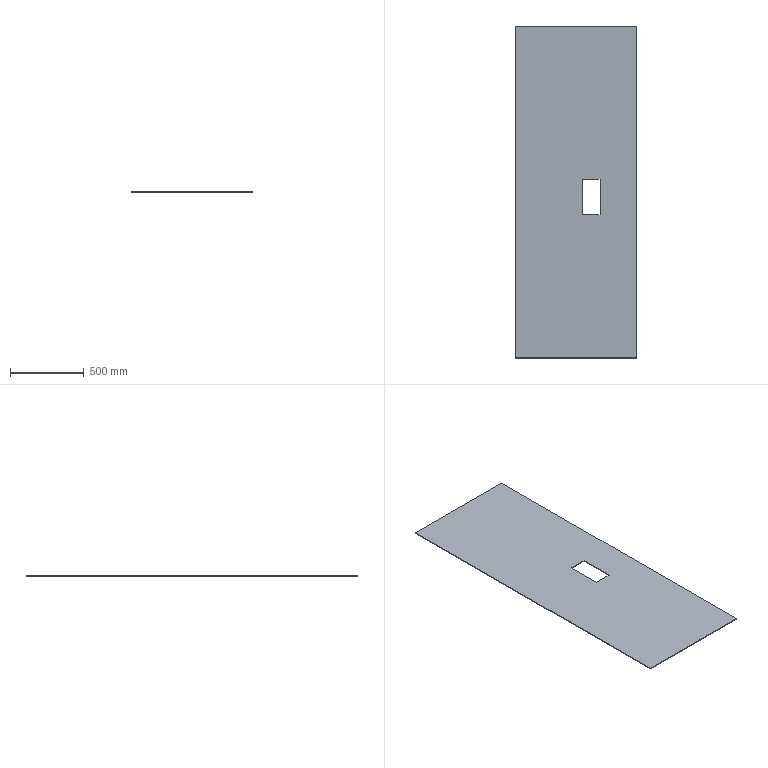Part | 1 solid | 10 faces | box 826 x 2252 x 5 mm | volume 9156760 mm3 | plane 10
STEP:
#1=CARTESIAN_POINT('',(-413.,1126.,5.));
#2=VERTEX_POINT('',#1);
#3=CARTESIAN_POINT('',(-413.,-1126.,5.));
#4=VERTEX_POINT('',#3);
#5=CARTESIAN_POINT('',(-413.,0.,5.));
#6=DIRECTION('',(0.,-1.,0.));
#7=VECTOR('',#6,1000.);
#8=LINE('',#5,#7);
#9=EDGE_CURVE('',#2,#4,#8,.T.);
#10=ORIENTED_EDGE('',*,*,#9,.T.);
#11=CARTESIAN_POINT('',(413.,-1126.,5.));
#12=VERTEX_POINT('',#11);
#13=CARTESIAN_POINT('',(0.,-1126.,5.));
#14=DIRECTION('',(1.,0.,0.));
#15=VECTOR('',#14,1000.);
#16=LINE('',#13,#15);
#17=EDGE_CURVE('',#4,#12,#16,.T.);
#18=ORIENTED_EDGE('',*,*,#17,.T.);
#19=CARTESIAN_POINT('',(413.,1126.,5.));
#20=VERTEX_POINT('',#19);
#21=CARTESIAN_POINT('',(413.,0.,5.));
#22=DIRECTION('',(0.,1.,0.));
#23=VECTOR('',#22,1000.);
#24=LINE('',#21,#23);
#25=EDGE_CURVE('',#12,#20,#24,.T.);
#26=ORIENTED_EDGE('',*,*,#25,.T.);
#27=CARTESIAN_POINT('',(0.,1126.,5.));
#28=DIRECTION('',(-1.,0.,0.));
#29=VECTOR('',#28,1000.);
#30=LINE('',#27,#29);
#31=EDGE_CURVE('',#20,#2,#30,.T.);
#32=ORIENTED_EDGE('',*,*,#31,.T.);
#33=EDGE_LOOP('',(#10,#18,#26,#32));
#34=FACE_OUTER_BOUND('',#33,.T.);
#35=CARTESIAN_POINT('',(163.,86.,5.));
#36=VERTEX_POINT('',#35);
#37=CARTESIAN_POINT('',(163.,-154.,5.));
#38=VERTEX_POINT('',#37);
#39=CARTESIAN_POINT('',(163.,0.,5.));
#40=DIRECTION('',(0.,-1.,0.));
#41=VECTOR('',#40,1000.);
#42=LINE('',#39,#41);
#43=EDGE_CURVE('',#36,#38,#42,.T.);
#44=ORIENTED_EDGE('',*,*,#43,.T.);
#45=CARTESIAN_POINT('',(43.,-154.,5.));
#46=VERTEX_POINT('',#45);
#47=CARTESIAN_POINT('',(0.,-154.,5.));
#48=DIRECTION('',(-1.,0.,0.));
#49=VECTOR('',#48,1000.);
#50=LINE('',#47,#49);
#51=EDGE_CURVE('',#38,#46,#50,.T.);
#52=ORIENTED_EDGE('',*,*,#51,.T.);
#53=CARTESIAN_POINT('',(43.,86.,5.));
#54=VERTEX_POINT('',#53);
#55=CARTESIAN_POINT('',(43.,0.,5.));
#56=DIRECTION('',(0.,1.,0.));
#57=VECTOR('',#56,1000.);
#58=LINE('',#55,#57);
#59=EDGE_CURVE('',#46,#54,#58,.T.);
#60=ORIENTED_EDGE('',*,*,#59,.T.);
#61=CARTESIAN_POINT('',(0.,86.,5.));
#62=DIRECTION('',(1.,0.,0.));
#63=VECTOR('',#62,1000.);
#64=LINE('',#61,#63);
#65=EDGE_CURVE('',#54,#36,#64,.T.);
#66=ORIENTED_EDGE('',*,*,#65,.T.);
#67=EDGE_LOOP('',(#44,#52,#60,#66));
#68=FACE_BOUND('',#67,.T.);
#69=CARTESIAN_POINT('',(0.,0.,5.));
#70=DIRECTION('',(0.,0.,1.));
#71=DIRECTION('',(1.,0.,0.));
#72=AXIS2_PLACEMENT_3D('',#69,#70,#71);
#73=PLANE('',#72);
#74=ADVANCED_FACE('',(#34,#68),#73,.T.);
#75=CARTESIAN_POINT('',(413.,-1126.,0.));
#76=VERTEX_POINT('',#75);
#77=CARTESIAN_POINT('',(413.,-1126.,5.));
#78=DIRECTION('',(0.,0.,-1.));
#79=VECTOR('',#78,1000.);
#80=LINE('',#77,#79);
#81=EDGE_CURVE('',#12,#76,#80,.T.);
#82=ORIENTED_EDGE('',*,*,#81,.F.);
#83=ORIENTED_EDGE('',*,*,#17,.F.);
#84=CARTESIAN_POINT('',(-413.,-1126.,0.));
#85=VERTEX_POINT('',#84);
#86=CARTESIAN_POINT('',(-413.,-1126.,5.));
#87=DIRECTION('',(0.,0.,1.));
#88=VECTOR('',#87,1000.);
#89=LINE('',#86,#88);
#90=EDGE_CURVE('',#85,#4,#89,.T.);
#91=ORIENTED_EDGE('',*,*,#90,.F.);
#92=CARTESIAN_POINT('',(-413.,-1126.,0.));
#93=DIRECTION('',(-1.,0.,0.));
#94=VECTOR('',#93,1000.);
#95=LINE('',#92,#94);
#96=EDGE_CURVE('',#76,#85,#95,.T.);
#97=ORIENTED_EDGE('',*,*,#96,.F.);
#98=EDGE_LOOP('',(#82,#83,#91,#97));
#99=FACE_OUTER_BOUND('',#98,.T.);
#100=CARTESIAN_POINT('',(-413.,-1126.,5.));
#101=DIRECTION('',(0.,1.,0.));
#102=DIRECTION('',(0.,0.,1.));
#103=AXIS2_PLACEMENT_3D('',#100,#101,#102);
#104=PLANE('',#103);
#105=ADVANCED_FACE('',(#99),#104,.F.);
#106=ORIENTED_EDGE('',*,*,#90,.T.);
#107=ORIENTED_EDGE('',*,*,#9,.F.);
#108=CARTESIAN_POINT('',(-413.,1126.,0.));
#109=VERTEX_POINT('',#108);
#110=CARTESIAN_POINT('',(-413.,1126.,5.));
#111=DIRECTION('',(0.,0.,1.));
#112=VECTOR('',#111,1000.);
#113=LINE('',#110,#112);
#114=EDGE_CURVE('',#109,#2,#113,.T.);
#115=ORIENTED_EDGE('',*,*,#114,.F.);
#116=CARTESIAN_POINT('',(-413.,1126.,0.));
#117=DIRECTION('',(0.,1.,0.));
#118=VECTOR('',#117,1000.);
#119=LINE('',#116,#118);
#120=EDGE_CURVE('',#85,#109,#119,.T.);
#121=ORIENTED_EDGE('',*,*,#120,.F.);
#122=EDGE_LOOP('',(#106,#107,#115,#121));
#123=FACE_OUTER_BOUND('',#122,.T.);
#124=CARTESIAN_POINT('',(-413.,1126.,5.));
#125=DIRECTION('',(1.,0.,0.));
#126=DIRECTION('',(0.,1.,0.));
#127=AXIS2_PLACEMENT_3D('',#124,#125,#126);
#128=PLANE('',#127);
#129=ADVANCED_FACE('',(#123),#128,.F.);
#130=ORIENTED_EDGE('',*,*,#114,.T.);
#131=ORIENTED_EDGE('',*,*,#31,.F.);
#132=CARTESIAN_POINT('',(413.,1126.,0.));
#133=VERTEX_POINT('',#132);
#134=CARTESIAN_POINT('',(413.,1126.,5.));
#135=DIRECTION('',(0.,0.,1.));
#136=VECTOR('',#135,1000.);
#137=LINE('',#134,#136);
#138=EDGE_CURVE('',#133,#20,#137,.T.);
#139=ORIENTED_EDGE('',*,*,#138,.F.);
#140=CARTESIAN_POINT('',(-413.,1126.,0.));
#141=DIRECTION('',(1.,0.,0.));
#142=VECTOR('',#141,1000.);
#143=LINE('',#140,#142);
#144=EDGE_CURVE('',#109,#133,#143,.T.);
#145=ORIENTED_EDGE('',*,*,#144,.F.);
#146=EDGE_LOOP('',(#130,#131,#139,#145));
#147=FACE_OUTER_BOUND('',#146,.T.);
#148=CARTESIAN_POINT('',(-413.,1126.,5.));
#149=DIRECTION('',(0.,-1.,0.));
#150=DIRECTION('',(0.,0.,-1.));
#151=AXIS2_PLACEMENT_3D('',#148,#149,#150);
#152=PLANE('',#151);
#153=ADVANCED_FACE('',(#147),#152,.F.);
#154=ORIENTED_EDGE('',*,*,#138,.T.);
#155=ORIENTED_EDGE('',*,*,#25,.F.);
#156=ORIENTED_EDGE('',*,*,#81,.T.);
#157=CARTESIAN_POINT('',(413.,1126.,0.));
#158=DIRECTION('',(0.,-1.,0.));
#159=VECTOR('',#158,1000.);
#160=LINE('',#157,#159);
#161=EDGE_CURVE('',#133,#76,#160,.T.);
#162=ORIENTED_EDGE('',*,*,#161,.F.);
#163=EDGE_LOOP('',(#154,#155,#156,#162));
#164=FACE_OUTER_BOUND('',#163,.T.);
#165=CARTESIAN_POINT('',(413.,1126.,5.));
#166=DIRECTION('',(-1.,0.,0.));
#167=DIRECTION('',(0.,-1.,0.));
#168=AXIS2_PLACEMENT_3D('',#165,#166,#167);
#169=PLANE('',#168);
#170=ADVANCED_FACE('',(#164),#169,.F.);
#171=CARTESIAN_POINT('',(163.,-154.,0.));
#172=VERTEX_POINT('',#171);
#173=CARTESIAN_POINT('',(163.,-154.,0.));
#174=DIRECTION('',(0.,0.,1.));
#175=VECTOR('',#174,1000.);
#176=LINE('',#173,#175);
#177=EDGE_CURVE('',#172,#38,#176,.T.);
#178=ORIENTED_EDGE('',*,*,#177,.F.);
#179=CARTESIAN_POINT('',(43.,-154.,0.));
#180=VERTEX_POINT('',#179);
#181=CARTESIAN_POINT('',(43.,-154.,0.));
#182=DIRECTION('',(1.,0.,0.));
#183=VECTOR('',#182,1000.);
#184=LINE('',#181,#183);
#185=EDGE_CURVE('',#180,#172,#184,.T.);
#186=ORIENTED_EDGE('',*,*,#185,.F.);
#187=CARTESIAN_POINT('',(43.,-154.,0.));
#188=DIRECTION('',(0.,0.,-1.));
#189=VECTOR('',#188,1000.);
#190=LINE('',#187,#189);
#191=EDGE_CURVE('',#46,#180,#190,.T.);
#192=ORIENTED_EDGE('',*,*,#191,.F.);
#193=ORIENTED_EDGE('',*,*,#51,.F.);
#194=EDGE_LOOP('',(#178,#186,#192,#193));
#195=FACE_OUTER_BOUND('',#194,.T.);
#196=CARTESIAN_POINT('',(43.,-154.,0.));
#197=DIRECTION('',(0.,-1.,0.));
#198=DIRECTION('',(0.,0.,-1.));
#199=AXIS2_PLACEMENT_3D('',#196,#197,#198);
#200=PLANE('',#199);
#201=ADVANCED_FACE('',(#195),#200,.F.);
#202=CARTESIAN_POINT('',(163.,86.,0.));
#203=VERTEX_POINT('',#202);
#204=CARTESIAN_POINT('',(163.,86.,0.));
#205=DIRECTION('',(0.,0.,1.));
#206=VECTOR('',#205,1000.);
#207=LINE('',#204,#206);
#208=EDGE_CURVE('',#203,#36,#207,.T.);
#209=ORIENTED_EDGE('',*,*,#208,.F.);
#210=CARTESIAN_POINT('',(163.,86.,0.));
#211=DIRECTION('',(0.,1.,0.));
#212=VECTOR('',#211,1000.);
#213=LINE('',#210,#212);
#214=EDGE_CURVE('',#172,#203,#213,.T.);
#215=ORIENTED_EDGE('',*,*,#214,.F.);
#216=ORIENTED_EDGE('',*,*,#177,.T.);
#217=ORIENTED_EDGE('',*,*,#43,.F.);
#218=EDGE_LOOP('',(#209,#215,#216,#217));
#219=FACE_OUTER_BOUND('',#218,.T.);
#220=CARTESIAN_POINT('',(163.,86.,0.));
#221=DIRECTION('',(1.,0.,0.));
#222=DIRECTION('',(0.,1.,0.));
#223=AXIS2_PLACEMENT_3D('',#220,#221,#222);
#224=PLANE('',#223);
#225=ADVANCED_FACE('',(#219),#224,.F.);
#226=CARTESIAN_POINT('',(43.,86.,0.));
#227=VERTEX_POINT('',#226);
#228=CARTESIAN_POINT('',(43.,86.,0.));
#229=DIRECTION('',(0.,0.,1.));
#230=VECTOR('',#229,1000.);
#231=LINE('',#228,#230);
#232=EDGE_CURVE('',#227,#54,#231,.T.);
#233=ORIENTED_EDGE('',*,*,#232,.F.);
#234=CARTESIAN_POINT('',(43.,86.,0.));
#235=DIRECTION('',(-1.,0.,0.));
#236=VECTOR('',#235,1000.);
#237=LINE('',#234,#236);
#238=EDGE_CURVE('',#203,#227,#237,.T.);
#239=ORIENTED_EDGE('',*,*,#238,.F.);
#240=ORIENTED_EDGE('',*,*,#208,.T.);
#241=ORIENTED_EDGE('',*,*,#65,.F.);
#242=EDGE_LOOP('',(#233,#239,#240,#241));
#243=FACE_OUTER_BOUND('',#242,.T.);
#244=CARTESIAN_POINT('',(43.,86.,0.));
#245=DIRECTION('',(0.,1.,0.));
#246=DIRECTION('',(0.,0.,1.));
#247=AXIS2_PLACEMENT_3D('',#244,#245,#246);
#248=PLANE('',#247);
#249=ADVANCED_FACE('',(#243),#248,.F.);
#250=ORIENTED_EDGE('',*,*,#191,.T.);
#251=CARTESIAN_POINT('',(43.,86.,0.));
#252=DIRECTION('',(0.,-1.,0.));
#253=VECTOR('',#252,1000.);
#254=LINE('',#251,#253);
#255=EDGE_CURVE('',#227,#180,#254,.T.);
#256=ORIENTED_EDGE('',*,*,#255,.F.);
#257=ORIENTED_EDGE('',*,*,#232,.T.);
#258=ORIENTED_EDGE('',*,*,#59,.F.);
#259=EDGE_LOOP('',(#250,#256,#257,#258));
#260=FACE_OUTER_BOUND('',#259,.T.);
#261=CARTESIAN_POINT('',(43.,86.,0.));
#262=DIRECTION('',(-1.,0.,0.));
#263=DIRECTION('',(0.,-1.,0.));
#264=AXIS2_PLACEMENT_3D('',#261,#262,#263);
#265=PLANE('',#264);
#266=ADVANCED_FACE('',(#260),#265,.F.);
#267=ORIENTED_EDGE('',*,*,#96,.T.);
#268=ORIENTED_EDGE('',*,*,#120,.T.);
#269=ORIENTED_EDGE('',*,*,#144,.T.);
#270=ORIENTED_EDGE('',*,*,#161,.T.);
#271=EDGE_LOOP('',(#267,#268,#269,#270));
#272=FACE_OUTER_BOUND('',#271,.T.);
#273=ORIENTED_EDGE('',*,*,#255,.T.);
#274=ORIENTED_EDGE('',*,*,#185,.T.);
#275=ORIENTED_EDGE('',*,*,#214,.T.);
#276=ORIENTED_EDGE('',*,*,#238,.T.);
#277=EDGE_LOOP('',(#273,#274,#275,#276));
#278=FACE_BOUND('',#277,.T.);
#279=CARTESIAN_POINT('',(0.,0.,0.));
#280=DIRECTION('',(0.,0.,1.));
#281=DIRECTION('',(1.,0.,0.));
#282=AXIS2_PLACEMENT_3D('',#279,#280,#281);
#283=PLANE('',#282);
#284=ADVANCED_FACE('',(#272,#278),#283,.F.);
#285=CLOSED_SHELL('',(#74,#105,#129,#153,#170,#201,#225,#249,#266,#284));
#286=MANIFOLD_SOLID_BREP('',#285);
#287=CARTESIAN_POINT('',(0.,0.,0.));
#288=DIRECTION('',(0.,0.,1.));
#289=DIRECTION('',(1.,0.,0.));
#290=AXIS2_PLACEMENT_3D('',#287,#288,#289);
#291=(LENGTH_UNIT()NAMED_UNIT(*)SI_UNIT(.MILLI.,.METRE.));
#292=UNCERTAINTY_MEASURE_WITH_UNIT(LENGTH_MEASURE(0.00001),#291,'','');
#293=(NAMED_UNIT(*)PLANE_ANGLE_UNIT()SI_UNIT($,.RADIAN.));
#294=(NAMED_UNIT(*)SI_UNIT($,.STERADIAN.)SOLID_ANGLE_UNIT());
#295=(GEOMETRIC_REPRESENTATION_CONTEXT(3)GLOBAL_UNCERTAINTY_ASSIGNED_CONTEXT((#292))GLOBAL_UNIT_ASSIGNED_CONTEXT((#291,#293,#294))REPRESENTATION_CONTEXT('',''));
#296=ADVANCED_BREP_SHAPE_REPRESENTATION('',(#286,#290),#295);